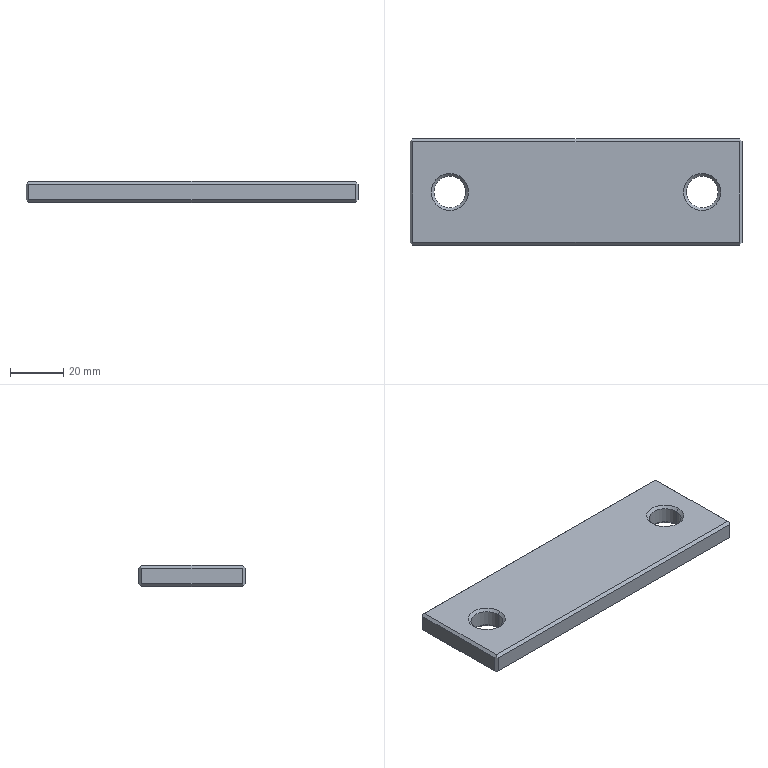Part | SolidWorks | features BaseBody 1 | 1 solid | 30 faces | box 125 x 40 x 8 mm | volume 37771 mm3 | plane 18 | cone 8 | cylinder 4 | commonest cylinder face diameters 12 x4
STEP:
#1=CARTESIAN_POINT('',(53.5,0.,1.));
#2=VERTEX_POINT('',#1);
#3=CARTESIAN_POINT('',(41.5,0.,1.));
#4=VERTEX_POINT('',#3);
#5=CARTESIAN_POINT('',(47.5,0.,1.));
#6=DIRECTION('',(0.,0.,-1.));
#7=DIRECTION('',(0.,-1.,0.));
#8=AXIS2_PLACEMENT_3D('',#5,#6,#7);
#9=CIRCLE('',#8,6.);
#10=EDGE_CURVE('',#2,#4,#9,.T.);
#11=ORIENTED_EDGE('',*,*,#10,.F.);
#12=CARTESIAN_POINT('',(54.5,0.,0.));
#13=VERTEX_POINT('',#12);
#14=CARTESIAN_POINT('',(54.5,0.,0.));
#15=DIRECTION('',(0.7071,0.,-0.7071));
#16=VECTOR('',#15,1000.);
#17=LINE('',#14,#16);
#18=EDGE_CURVE('',#2,#13,#17,.T.);
#19=ORIENTED_EDGE('',*,*,#18,.T.);
#20=CARTESIAN_POINT('',(40.5,0.,0.));
#21=VERTEX_POINT('',#20);
#22=CARTESIAN_POINT('',(47.5,0.,0.));
#23=DIRECTION('',(0.,0.,-1.));
#24=DIRECTION('',(-1.,0.,0.));
#25=AXIS2_PLACEMENT_3D('',#22,#23,#24);
#26=CIRCLE('',#25,7.);
#27=EDGE_CURVE('',#13,#21,#26,.T.);
#28=ORIENTED_EDGE('',*,*,#27,.T.);
#29=CARTESIAN_POINT('',(40.5,0.,0.));
#30=DIRECTION('',(-0.7071,0.,-0.7071));
#31=VECTOR('',#30,1000.);
#32=LINE('',#29,#31);
#33=EDGE_CURVE('',#4,#21,#32,.T.);
#34=ORIENTED_EDGE('',*,*,#33,.F.);
#35=EDGE_LOOP('',(#11,#19,#28,#34));
#36=FACE_OUTER_BOUND('',#35,.T.);
#37=CARTESIAN_POINT('',(47.5,0.,0.));
#38=DIRECTION('',(0.,0.,-1.));
#39=DIRECTION('',(-1.,0.,0.));
#40=AXIS2_PLACEMENT_3D('',#37,#38,#39);
#41=CONICAL_SURFACE('',#40,7.,0.7854);
#42=ADVANCED_FACE('',(#36),#41,.F.);
#43=CARTESIAN_POINT('',(-41.5,0.,1.));
#44=VERTEX_POINT('',#43);
#45=CARTESIAN_POINT('',(-53.5,0.,1.));
#46=VERTEX_POINT('',#45);
#47=CARTESIAN_POINT('',(-47.5,0.,1.));
#48=DIRECTION('',(0.,0.,-1.));
#49=DIRECTION('',(0.,-1.,0.));
#50=AXIS2_PLACEMENT_3D('',#47,#48,#49);
#51=CIRCLE('',#50,6.);
#52=EDGE_CURVE('',#44,#46,#51,.T.);
#53=ORIENTED_EDGE('',*,*,#52,.F.);
#54=CARTESIAN_POINT('',(-40.5,0.,0.));
#55=VERTEX_POINT('',#54);
#56=CARTESIAN_POINT('',(-40.5,0.,0.));
#57=DIRECTION('',(0.7071,0.,-0.7071));
#58=VECTOR('',#57,1000.);
#59=LINE('',#56,#58);
#60=EDGE_CURVE('',#44,#55,#59,.T.);
#61=ORIENTED_EDGE('',*,*,#60,.T.);
#62=CARTESIAN_POINT('',(-54.5,0.,0.));
#63=VERTEX_POINT('',#62);
#64=CARTESIAN_POINT('',(-47.5,0.,0.));
#65=DIRECTION('',(0.,0.,-1.));
#66=DIRECTION('',(-1.,0.,0.));
#67=AXIS2_PLACEMENT_3D('',#64,#65,#66);
#68=CIRCLE('',#67,7.);
#69=EDGE_CURVE('',#55,#63,#68,.T.);
#70=ORIENTED_EDGE('',*,*,#69,.T.);
#71=CARTESIAN_POINT('',(-54.5,0.,0.));
#72=DIRECTION('',(-0.7071,0.,-0.7071));
#73=VECTOR('',#72,1000.);
#74=LINE('',#71,#73);
#75=EDGE_CURVE('',#46,#63,#74,.T.);
#76=ORIENTED_EDGE('',*,*,#75,.F.);
#77=EDGE_LOOP('',(#53,#61,#70,#76));
#78=FACE_OUTER_BOUND('',#77,.T.);
#79=CARTESIAN_POINT('',(-47.5,0.,0.));
#80=DIRECTION('',(0.,0.,-1.));
#81=DIRECTION('',(-1.,0.,0.));
#82=AXIS2_PLACEMENT_3D('',#79,#80,#81);
#83=CONICAL_SURFACE('',#82,7.,0.7854);
#84=ADVANCED_FACE('',(#78),#83,.F.);
#85=CARTESIAN_POINT('',(53.5,0.,7.));
#86=VERTEX_POINT('',#85);
#87=CARTESIAN_POINT('',(41.5,0.,7.));
#88=VERTEX_POINT('',#87);
#89=CARTESIAN_POINT('',(47.5,0.,7.));
#90=DIRECTION('',(0.,0.,-1.));
#91=DIRECTION('',(-1.,0.,0.));
#92=AXIS2_PLACEMENT_3D('',#89,#90,#91);
#93=CIRCLE('',#92,6.);
#94=EDGE_CURVE('',#86,#88,#93,.T.);
#95=ORIENTED_EDGE('',*,*,#94,.F.);
#96=CARTESIAN_POINT('',(53.5,0.,8.));
#97=DIRECTION('',(0.,0.,-1.));
#98=VECTOR('',#97,1000.);
#99=LINE('',#96,#98);
#100=EDGE_CURVE('',#86,#2,#99,.T.);
#101=ORIENTED_EDGE('',*,*,#100,.T.);
#102=ORIENTED_EDGE('',*,*,#10,.T.);
#103=CARTESIAN_POINT('',(41.5,0.,8.));
#104=DIRECTION('',(0.,0.,-1.));
#105=VECTOR('',#104,1000.);
#106=LINE('',#103,#105);
#107=EDGE_CURVE('',#88,#4,#106,.T.);
#108=ORIENTED_EDGE('',*,*,#107,.F.);
#109=EDGE_LOOP('',(#95,#101,#102,#108));
#110=FACE_OUTER_BOUND('',#109,.T.);
#111=CARTESIAN_POINT('',(47.5,0.,8.));
#112=DIRECTION('',(0.,0.,-1.));
#113=DIRECTION('',(-1.,0.,0.));
#114=AXIS2_PLACEMENT_3D('',#111,#112,#113);
#115=CYLINDRICAL_SURFACE('',#114,6.);
#116=ADVANCED_FACE('',(#110),#115,.F.);
#117=CARTESIAN_POINT('',(-41.5,0.,7.));
#118=VERTEX_POINT('',#117);
#119=CARTESIAN_POINT('',(-53.5,0.,7.));
#120=VERTEX_POINT('',#119);
#121=CARTESIAN_POINT('',(-47.5,0.,7.));
#122=DIRECTION('',(0.,0.,-1.));
#123=DIRECTION('',(-1.,0.,0.));
#124=AXIS2_PLACEMENT_3D('',#121,#122,#123);
#125=CIRCLE('',#124,6.);
#126=EDGE_CURVE('',#118,#120,#125,.T.);
#127=ORIENTED_EDGE('',*,*,#126,.F.);
#128=CARTESIAN_POINT('',(-41.5,0.,8.));
#129=DIRECTION('',(0.,0.,-1.));
#130=VECTOR('',#129,1000.);
#131=LINE('',#128,#130);
#132=EDGE_CURVE('',#118,#44,#131,.T.);
#133=ORIENTED_EDGE('',*,*,#132,.T.);
#134=ORIENTED_EDGE('',*,*,#52,.T.);
#135=CARTESIAN_POINT('',(-53.5,0.,8.));
#136=DIRECTION('',(0.,0.,-1.));
#137=VECTOR('',#136,1000.);
#138=LINE('',#135,#137);
#139=EDGE_CURVE('',#120,#46,#138,.T.);
#140=ORIENTED_EDGE('',*,*,#139,.F.);
#141=EDGE_LOOP('',(#127,#133,#134,#140));
#142=FACE_OUTER_BOUND('',#141,.T.);
#143=CARTESIAN_POINT('',(-47.5,0.,8.));
#144=DIRECTION('',(0.,0.,-1.));
#145=DIRECTION('',(-1.,0.,0.));
#146=AXIS2_PLACEMENT_3D('',#143,#144,#145);
#147=CYLINDRICAL_SURFACE('',#146,6.);
#148=ADVANCED_FACE('',(#142),#147,.F.);
#149=ORIENTED_EDGE('',*,*,#94,.T.);
#150=CARTESIAN_POINT('',(40.5,0.,8.));
#151=VERTEX_POINT('',#150);
#152=CARTESIAN_POINT('',(40.5,0.,8.));
#153=DIRECTION('',(-0.7071,0.,0.7071));
#154=VECTOR('',#153,1000.);
#155=LINE('',#152,#154);
#156=EDGE_CURVE('',#88,#151,#155,.T.);
#157=ORIENTED_EDGE('',*,*,#156,.T.);
#158=CARTESIAN_POINT('',(54.5,0.,8.));
#159=VERTEX_POINT('',#158);
#160=CARTESIAN_POINT('',(47.5,0.,8.));
#161=DIRECTION('',(0.,0.,-1.));
#162=DIRECTION('',(1.,0.,0.));
#163=AXIS2_PLACEMENT_3D('',#160,#161,#162);
#164=CIRCLE('',#163,7.);
#165=EDGE_CURVE('',#159,#151,#164,.T.);
#166=ORIENTED_EDGE('',*,*,#165,.F.);
#167=CARTESIAN_POINT('',(54.5,0.,8.));
#168=DIRECTION('',(0.7071,0.,0.7071));
#169=VECTOR('',#168,1000.);
#170=LINE('',#167,#169);
#171=EDGE_CURVE('',#86,#159,#170,.T.);
#172=ORIENTED_EDGE('',*,*,#171,.F.);
#173=EDGE_LOOP('',(#149,#157,#166,#172));
#174=FACE_OUTER_BOUND('',#173,.T.);
#175=CARTESIAN_POINT('',(47.5,0.,8.));
#176=DIRECTION('',(0.,0.,1.));
#177=DIRECTION('',(1.,0.,0.));
#178=AXIS2_PLACEMENT_3D('',#175,#176,#177);
#179=CONICAL_SURFACE('',#178,7.,0.7854);
#180=ADVANCED_FACE('',(#174),#179,.F.);
#181=ORIENTED_EDGE('',*,*,#126,.T.);
#182=CARTESIAN_POINT('',(-54.5,0.,8.));
#183=VERTEX_POINT('',#182);
#184=CARTESIAN_POINT('',(-54.5,0.,8.));
#185=DIRECTION('',(-0.7071,0.,0.7071));
#186=VECTOR('',#185,1000.);
#187=LINE('',#184,#186);
#188=EDGE_CURVE('',#120,#183,#187,.T.);
#189=ORIENTED_EDGE('',*,*,#188,.T.);
#190=CARTESIAN_POINT('',(-40.5,0.,8.));
#191=VERTEX_POINT('',#190);
#192=CARTESIAN_POINT('',(-47.5,0.,8.));
#193=DIRECTION('',(0.,0.,-1.));
#194=DIRECTION('',(1.,0.,0.));
#195=AXIS2_PLACEMENT_3D('',#192,#193,#194);
#196=CIRCLE('',#195,7.);
#197=EDGE_CURVE('',#191,#183,#196,.T.);
#198=ORIENTED_EDGE('',*,*,#197,.F.);
#199=CARTESIAN_POINT('',(-40.5,0.,8.));
#200=DIRECTION('',(0.7071,0.,0.7071));
#201=VECTOR('',#200,1000.);
#202=LINE('',#199,#201);
#203=EDGE_CURVE('',#118,#191,#202,.T.);
#204=ORIENTED_EDGE('',*,*,#203,.F.);
#205=EDGE_LOOP('',(#181,#189,#198,#204));
#206=FACE_OUTER_BOUND('',#205,.T.);
#207=CARTESIAN_POINT('',(-47.5,0.,8.));
#208=DIRECTION('',(0.,0.,1.));
#209=DIRECTION('',(1.,0.,0.));
#210=AXIS2_PLACEMENT_3D('',#207,#208,#209);
#211=CONICAL_SURFACE('',#210,7.,0.7854);
#212=ADVANCED_FACE('',(#206),#211,.F.);
#213=CARTESIAN_POINT('',(47.5,0.,0.));
#214=DIRECTION('',(0.,0.,-1.));
#215=DIRECTION('',(-1.,0.,0.));
#216=AXIS2_PLACEMENT_3D('',#213,#214,#215);
#217=CIRCLE('',#216,7.);
#218=EDGE_CURVE('',#21,#13,#217,.T.);
#219=ORIENTED_EDGE('',*,*,#218,.F.);
#220=ORIENTED_EDGE('',*,*,#27,.F.);
#221=EDGE_LOOP('',(#219,#220));
#222=FACE_BOUND('',#221,.T.);
#223=CARTESIAN_POINT('',(-47.5,0.,0.));
#224=DIRECTION('',(0.,0.,-1.));
#225=DIRECTION('',(-1.,0.,0.));
#226=AXIS2_PLACEMENT_3D('',#223,#224,#225);
#227=CIRCLE('',#226,7.);
#228=EDGE_CURVE('',#63,#55,#227,.T.);
#229=ORIENTED_EDGE('',*,*,#228,.F.);
#230=ORIENTED_EDGE('',*,*,#69,.F.);
#231=EDGE_LOOP('',(#229,#230));
#232=FACE_BOUND('',#231,.T.);
#233=CARTESIAN_POINT('',(-61.5,-19.,0.));
#234=VERTEX_POINT('',#233);
#235=CARTESIAN_POINT('',(61.5,-19.,0.));
#236=VERTEX_POINT('',#235);
#237=CARTESIAN_POINT('',(0.,-19.,0.));
#238=DIRECTION('',(1.,0.,0.));
#239=VECTOR('',#238,1000.);
#240=LINE('',#237,#239);
#241=EDGE_CURVE('',#234,#236,#240,.T.);
#242=ORIENTED_EDGE('',*,*,#241,.F.);
#243=CARTESIAN_POINT('',(-61.5,19.,0.));
#244=VERTEX_POINT('',#243);
#245=CARTESIAN_POINT('',(-61.5,0.,0.));
#246=DIRECTION('',(0.,-1.,0.));
#247=VECTOR('',#246,1000.);
#248=LINE('',#245,#247);
#249=EDGE_CURVE('',#244,#234,#248,.T.);
#250=ORIENTED_EDGE('',*,*,#249,.F.);
#251=CARTESIAN_POINT('',(61.5,19.,0.));
#252=VERTEX_POINT('',#251);
#253=CARTESIAN_POINT('',(0.,19.,0.));
#254=DIRECTION('',(-1.,0.,0.));
#255=VECTOR('',#254,1000.);
#256=LINE('',#253,#255);
#257=EDGE_CURVE('',#252,#244,#256,.T.);
#258=ORIENTED_EDGE('',*,*,#257,.F.);
#259=CARTESIAN_POINT('',(61.5,0.,0.));
#260=DIRECTION('',(0.,1.,0.));
#261=VECTOR('',#260,1000.);
#262=LINE('',#259,#261);
#263=EDGE_CURVE('',#236,#252,#262,.T.);
#264=ORIENTED_EDGE('',*,*,#263,.F.);
#265=EDGE_LOOP('',(#242,#250,#258,#264));
#266=FACE_OUTER_BOUND('',#265,.T.);
#267=CARTESIAN_POINT('',(0.,0.,0.));
#268=DIRECTION('',(0.,0.,1.));
#269=DIRECTION('',(1.,0.,0.));
#270=AXIS2_PLACEMENT_3D('',#267,#268,#269);
#271=PLANE('',#270);
#272=ADVANCED_FACE('',(#222,#232,#266),#271,.F.);
#273=ORIENTED_EDGE('',*,*,#18,.F.);
#274=CARTESIAN_POINT('',(47.5,0.,1.));
#275=DIRECTION('',(0.,0.,-1.));
#276=DIRECTION('',(0.,-1.,0.));
#277=AXIS2_PLACEMENT_3D('',#274,#275,#276);
#278=CIRCLE('',#277,6.);
#279=EDGE_CURVE('',#4,#2,#278,.T.);
#280=ORIENTED_EDGE('',*,*,#279,.F.);
#281=ORIENTED_EDGE('',*,*,#33,.T.);
#282=ORIENTED_EDGE('',*,*,#218,.T.);
#283=EDGE_LOOP('',(#273,#280,#281,#282));
#284=FACE_OUTER_BOUND('',#283,.T.);
#285=CARTESIAN_POINT('',(47.5,0.,0.));
#286=DIRECTION('',(0.,0.,-1.));
#287=DIRECTION('',(-1.,0.,0.));
#288=AXIS2_PLACEMENT_3D('',#285,#286,#287);
#289=CONICAL_SURFACE('',#288,7.,0.7854);
#290=ADVANCED_FACE('',(#284),#289,.F.);
#291=ORIENTED_EDGE('',*,*,#60,.F.);
#292=CARTESIAN_POINT('',(-47.5,0.,1.));
#293=DIRECTION('',(0.,0.,-1.));
#294=DIRECTION('',(0.,-1.,0.));
#295=AXIS2_PLACEMENT_3D('',#292,#293,#294);
#296=CIRCLE('',#295,6.);
#297=EDGE_CURVE('',#46,#44,#296,.T.);
#298=ORIENTED_EDGE('',*,*,#297,.F.);
#299=ORIENTED_EDGE('',*,*,#75,.T.);
#300=ORIENTED_EDGE('',*,*,#228,.T.);
#301=EDGE_LOOP('',(#291,#298,#299,#300));
#302=FACE_OUTER_BOUND('',#301,.T.);
#303=CARTESIAN_POINT('',(-47.5,0.,0.));
#304=DIRECTION('',(0.,0.,-1.));
#305=DIRECTION('',(-1.,0.,0.));
#306=AXIS2_PLACEMENT_3D('',#303,#304,#305);
#307=CONICAL_SURFACE('',#306,7.,0.7854);
#308=ADVANCED_FACE('',(#302),#307,.F.);
#309=CARTESIAN_POINT('',(62.,-19.5,0.5));
#310=VERTEX_POINT('',#309);
#311=CARTESIAN_POINT('',(62.,-19.5,0.5));
#312=DIRECTION('',(-0.5774,0.5774,-0.5774));
#313=VECTOR('',#312,1000.);
#314=LINE('',#311,#313);
#315=EDGE_CURVE('',#310,#236,#314,.T.);
#316=ORIENTED_EDGE('',*,*,#315,.T.);
#317=ORIENTED_EDGE('',*,*,#263,.T.);
#318=CARTESIAN_POINT('',(62.,19.5,0.5));
#319=VERTEX_POINT('',#318);
#320=CARTESIAN_POINT('',(61.5,19.,0.));
#321=DIRECTION('',(0.5774,0.5774,0.5774));
#322=VECTOR('',#321,1000.);
#323=LINE('',#320,#322);
#324=EDGE_CURVE('',#252,#319,#323,.T.);
#325=ORIENTED_EDGE('',*,*,#324,.T.);
#326=CARTESIAN_POINT('',(62.5,19.,1.));
#327=VERTEX_POINT('',#326);
#328=CARTESIAN_POINT('',(62.5,19.,1.));
#329=DIRECTION('',(-0.5774,0.5774,-0.5774));
#330=VECTOR('',#329,1000.);
#331=LINE('',#328,#330);
#332=EDGE_CURVE('',#327,#319,#331,.T.);
#333=ORIENTED_EDGE('',*,*,#332,.F.);
#334=CARTESIAN_POINT('',(62.5,-19.,1.));
#335=VERTEX_POINT('',#334);
#336=CARTESIAN_POINT('',(62.5,0.,1.));
#337=DIRECTION('',(0.,-1.,0.));
#338=VECTOR('',#337,1000.);
#339=LINE('',#336,#338);
#340=EDGE_CURVE('',#327,#335,#339,.T.);
#341=ORIENTED_EDGE('',*,*,#340,.T.);
#342=CARTESIAN_POINT('',(62.,-19.5,0.5));
#343=DIRECTION('',(0.5774,0.5774,0.5774));
#344=VECTOR('',#343,1000.);
#345=LINE('',#342,#344);
#346=EDGE_CURVE('',#310,#335,#345,.T.);
#347=ORIENTED_EDGE('',*,*,#346,.F.);
#348=EDGE_LOOP('',(#316,#317,#325,#333,#341,#347));
#349=FACE_OUTER_BOUND('',#348,.T.);
#350=CARTESIAN_POINT('',(62.,0.,0.5));
#351=DIRECTION('',(0.7071,0.,-0.7071));
#352=DIRECTION('',(-0.7071,0.,-0.7071));
#353=AXIS2_PLACEMENT_3D('',#350,#351,#352);
#354=PLANE('',#353);
#355=ADVANCED_FACE('',(#349),#354,.T.);
#356=CARTESIAN_POINT('',(-62.,-19.5,0.5));
#357=VERTEX_POINT('',#356);
#358=CARTESIAN_POINT('',(-62.,-19.5,0.5));
#359=DIRECTION('',(0.5774,0.5774,-0.5774));
#360=VECTOR('',#359,1000.);
#361=LINE('',#358,#360);
#362=EDGE_CURVE('',#357,#234,#361,.T.);
#363=ORIENTED_EDGE('',*,*,#362,.T.);
#364=ORIENTED_EDGE('',*,*,#241,.T.);
#365=ORIENTED_EDGE('',*,*,#315,.F.);
#366=CARTESIAN_POINT('',(61.5,-20.,1.));
#367=VERTEX_POINT('',#366);
#368=CARTESIAN_POINT('',(61.5,-20.,1.));
#369=DIRECTION('',(0.5774,0.5774,-0.5774));
#370=VECTOR('',#369,1000.);
#371=LINE('',#368,#370);
#372=EDGE_CURVE('',#367,#310,#371,.T.);
#373=ORIENTED_EDGE('',*,*,#372,.F.);
#374=CARTESIAN_POINT('',(-61.5,-20.,1.));
#375=VERTEX_POINT('',#374);
#376=CARTESIAN_POINT('',(0.,-20.,1.));
#377=DIRECTION('',(-1.,0.,0.));
#378=VECTOR('',#377,1000.);
#379=LINE('',#376,#378);
#380=EDGE_CURVE('',#367,#375,#379,.T.);
#381=ORIENTED_EDGE('',*,*,#380,.T.);
#382=CARTESIAN_POINT('',(-62.,-19.5,0.5));
#383=DIRECTION('',(0.5774,-0.5774,0.5774));
#384=VECTOR('',#383,1000.);
#385=LINE('',#382,#384);
#386=EDGE_CURVE('',#357,#375,#385,.T.);
#387=ORIENTED_EDGE('',*,*,#386,.F.);
#388=EDGE_LOOP('',(#363,#364,#365,#373,#381,#387));
#389=FACE_OUTER_BOUND('',#388,.T.);
#390=CARTESIAN_POINT('',(0.,-19.5,0.5));
#391=DIRECTION('',(0.,-0.7071,-0.7071));
#392=DIRECTION('',(0.,0.7071,-0.7071));
#393=AXIS2_PLACEMENT_3D('',#390,#391,#392);
#394=PLANE('',#393);
#395=ADVANCED_FACE('',(#389),#394,.T.);
#396=CARTESIAN_POINT('',(-62.5,-19.,1.));
#397=VERTEX_POINT('',#396);
#398=CARTESIAN_POINT('',(-62.5,-19.,1.));
#399=DIRECTION('',(0.5774,-0.5774,-0.5774));
#400=VECTOR('',#399,1000.);
#401=LINE('',#398,#400);
#402=EDGE_CURVE('',#397,#357,#401,.T.);
#403=ORIENTED_EDGE('',*,*,#402,.F.);
#404=CARTESIAN_POINT('',(-62.5,19.,1.));
#405=VERTEX_POINT('',#404);
#406=CARTESIAN_POINT('',(-62.5,0.,1.));
#407=DIRECTION('',(0.,1.,0.));
#408=VECTOR('',#407,1000.);
#409=LINE('',#406,#408);
#410=EDGE_CURVE('',#397,#405,#409,.T.);
#411=ORIENTED_EDGE('',*,*,#410,.T.);
#412=CARTESIAN_POINT('',(-62.,19.5,0.5));
#413=VERTEX_POINT('',#412);
#414=CARTESIAN_POINT('',(-62.,19.5,0.5));
#415=DIRECTION('',(-0.5774,-0.5774,0.5774));
#416=VECTOR('',#415,1000.);
#417=LINE('',#414,#416);
#418=EDGE_CURVE('',#413,#405,#417,.T.);
#419=ORIENTED_EDGE('',*,*,#418,.F.);
#420=CARTESIAN_POINT('',(-62.,19.5,0.5));
#421=DIRECTION('',(0.5774,-0.5774,-0.5774));
#422=VECTOR('',#421,1000.);
#423=LINE('',#420,#422);
#424=EDGE_CURVE('',#413,#244,#423,.T.);
#425=ORIENTED_EDGE('',*,*,#424,.T.);
#426=ORIENTED_EDGE('',*,*,#249,.T.);
#427=ORIENTED_EDGE('',*,*,#362,.F.);
#428=EDGE_LOOP('',(#403,#411,#419,#425,#426,#427));
#429=FACE_OUTER_BOUND('',#428,.T.);
#430=CARTESIAN_POINT('',(-62.,0.,0.5));
#431=DIRECTION('',(-0.7071,0.,-0.7071));
#432=DIRECTION('',(-0.7071,0.,0.7071));
#433=AXIS2_PLACEMENT_3D('',#430,#431,#432);
#434=PLANE('',#433);
#435=ADVANCED_FACE('',(#429),#434,.T.);
#436=CARTESIAN_POINT('',(-61.5,20.,1.));
#437=VERTEX_POINT('',#436);
#438=CARTESIAN_POINT('',(-61.5,20.,1.));
#439=DIRECTION('',(-0.5774,-0.5774,-0.5774));
#440=VECTOR('',#439,1000.);
#441=LINE('',#438,#440);
#442=EDGE_CURVE('',#437,#413,#441,.T.);
#443=ORIENTED_EDGE('',*,*,#442,.F.);
#444=CARTESIAN_POINT('',(61.5,20.,1.));
#445=VERTEX_POINT('',#444);
#446=CARTESIAN_POINT('',(0.,20.,1.));
#447=DIRECTION('',(1.,0.,0.));
#448=VECTOR('',#447,1000.);
#449=LINE('',#446,#448);
#450=EDGE_CURVE('',#437,#445,#449,.T.);
#451=ORIENTED_EDGE('',*,*,#450,.T.);
#452=CARTESIAN_POINT('',(62.,19.5,0.5));
#453=DIRECTION('',(-0.5774,0.5774,0.5774));
#454=VECTOR('',#453,1000.);
#455=LINE('',#452,#454);
#456=EDGE_CURVE('',#319,#445,#455,.T.);
#457=ORIENTED_EDGE('',*,*,#456,.F.);
#458=ORIENTED_EDGE('',*,*,#324,.F.);
#459=ORIENTED_EDGE('',*,*,#257,.T.);
#460=ORIENTED_EDGE('',*,*,#424,.F.);
#461=EDGE_LOOP('',(#443,#451,#457,#458,#459,#460));
#462=FACE_OUTER_BOUND('',#461,.T.);
#463=CARTESIAN_POINT('',(0.,19.5,0.5));
#464=DIRECTION('',(0.,0.7071,-0.7071));
#465=DIRECTION('',(0.,0.7071,0.7071));
#466=AXIS2_PLACEMENT_3D('',#463,#464,#465);
#467=PLANE('',#466);
#468=ADVANCED_FACE('',(#462),#467,.T.);
#469=ORIENTED_EDGE('',*,*,#100,.F.);
#470=CARTESIAN_POINT('',(47.5,0.,7.));
#471=DIRECTION('',(0.,0.,-1.));
#472=DIRECTION('',(-1.,0.,0.));
#473=AXIS2_PLACEMENT_3D('',#470,#471,#472);
#474=CIRCLE('',#473,6.);
#475=EDGE_CURVE('',#88,#86,#474,.T.);
#476=ORIENTED_EDGE('',*,*,#475,.F.);
#477=ORIENTED_EDGE('',*,*,#107,.T.);
#478=ORIENTED_EDGE('',*,*,#279,.T.);
#479=EDGE_LOOP('',(#469,#476,#477,#478));
#480=FACE_OUTER_BOUND('',#479,.T.);
#481=CARTESIAN_POINT('',(47.5,0.,8.));
#482=DIRECTION('',(0.,0.,-1.));
#483=DIRECTION('',(-1.,0.,0.));
#484=AXIS2_PLACEMENT_3D('',#481,#482,#483);
#485=CYLINDRICAL_SURFACE('',#484,6.);
#486=ADVANCED_FACE('',(#480),#485,.F.);
#487=ORIENTED_EDGE('',*,*,#132,.F.);
#488=CARTESIAN_POINT('',(-47.5,0.,7.));
#489=DIRECTION('',(0.,0.,-1.));
#490=DIRECTION('',(-1.,0.,0.));
#491=AXIS2_PLACEMENT_3D('',#488,#489,#490);
#492=CIRCLE('',#491,6.);
#493=EDGE_CURVE('',#120,#118,#492,.T.);
#494=ORIENTED_EDGE('',*,*,#493,.F.);
#495=ORIENTED_EDGE('',*,*,#139,.T.);
#496=ORIENTED_EDGE('',*,*,#297,.T.);
#497=EDGE_LOOP('',(#487,#494,#495,#496));
#498=FACE_OUTER_BOUND('',#497,.T.);
#499=CARTESIAN_POINT('',(-47.5,0.,8.));
#500=DIRECTION('',(0.,0.,-1.));
#501=DIRECTION('',(-1.,0.,0.));
#502=AXIS2_PLACEMENT_3D('',#499,#500,#501);
#503=CYLINDRICAL_SURFACE('',#502,6.);
#504=ADVANCED_FACE('',(#498),#503,.F.);
#505=CARTESIAN_POINT('',(62.5,19.,7.));
#506=VERTEX_POINT('',#505);
#507=CARTESIAN_POINT('',(62.5,-19.,7.));
#508=VERTEX_POINT('',#507);
#509=CARTESIAN_POINT('',(62.5,-20.,7.));
#510=DIRECTION('',(0.,-1.,0.));
#511=VECTOR('',#510,1000.);
#512=LINE('',#509,#511);
#513=EDGE_CURVE('',#506,#508,#512,.T.);
#514=ORIENTED_EDGE('',*,*,#513,.T.);
#515=CARTESIAN_POINT('',(62.5,-19.,0.));
#516=DIRECTION('',(0.,0.,-1.));
#517=VECTOR('',#516,1000.);
#518=LINE('',#515,#517);
#519=EDGE_CURVE('',#508,#335,#518,.T.);
#520=ORIENTED_EDGE('',*,*,#519,.T.);
#521=ORIENTED_EDGE('',*,*,#340,.F.);
#522=CARTESIAN_POINT('',(62.5,19.,0.));
#523=DIRECTION('',(0.,0.,1.));
#524=VECTOR('',#523,1000.);
#525=LINE('',#522,#524);
#526=EDGE_CURVE('',#327,#506,#525,.T.);
#527=ORIENTED_EDGE('',*,*,#526,.T.);
#528=EDGE_LOOP('',(#514,#520,#521,#527));
#529=FACE_OUTER_BOUND('',#528,.T.);
#530=CARTESIAN_POINT('',(62.5,-20.,0.));
#531=DIRECTION('',(1.,0.,0.));
#532=DIRECTION('',(0.,0.,-1.));
#533=AXIS2_PLACEMENT_3D('',#530,#531,#532);
#534=PLANE('',#533);
#535=ADVANCED_FACE('',(#529),#534,.T.);
#536=CARTESIAN_POINT('',(61.5,-20.,7.));
#537=VERTEX_POINT('',#536);
#538=CARTESIAN_POINT('',(-61.5,-20.,7.));
#539=VERTEX_POINT('',#538);
#540=CARTESIAN_POINT('',(-62.5,-20.,7.));
#541=DIRECTION('',(-1.,0.,0.));
#542=VECTOR('',#541,1000.);
#543=LINE('',#540,#542);
#544=EDGE_CURVE('',#537,#539,#543,.T.);
#545=ORIENTED_EDGE('',*,*,#544,.T.);
#546=CARTESIAN_POINT('',(-61.5,-20.,0.));
#547=DIRECTION('',(0.,0.,-1.));
#548=VECTOR('',#547,1000.);
#549=LINE('',#546,#548);
#550=EDGE_CURVE('',#539,#375,#549,.T.);
#551=ORIENTED_EDGE('',*,*,#550,.T.);
#552=ORIENTED_EDGE('',*,*,#380,.F.);
#553=CARTESIAN_POINT('',(61.5,-20.,0.));
#554=DIRECTION('',(0.,0.,1.));
#555=VECTOR('',#554,1000.);
#556=LINE('',#553,#555);
#557=EDGE_CURVE('',#367,#537,#556,.T.);
#558=ORIENTED_EDGE('',*,*,#557,.T.);
#559=EDGE_LOOP('',(#545,#551,#552,#558));
#560=FACE_OUTER_BOUND('',#559,.T.);
#561=CARTESIAN_POINT('',(-62.5,-20.,0.));
#562=DIRECTION('',(0.,-1.,0.));
#563=DIRECTION('',(0.,0.,-1.));
#564=AXIS2_PLACEMENT_3D('',#561,#562,#563);
#565=PLANE('',#564);
#566=ADVANCED_FACE('',(#560),#565,.T.);
#567=CARTESIAN_POINT('',(-62.5,-19.,7.));
#568=VERTEX_POINT('',#567);
#569=CARTESIAN_POINT('',(-62.5,-19.,0.));
#570=DIRECTION('',(0.,0.,1.));
#571=VECTOR('',#570,1000.);
#572=LINE('',#569,#571);
#573=EDGE_CURVE('',#397,#568,#572,.T.);
#574=ORIENTED_EDGE('',*,*,#573,.T.);
#575=CARTESIAN_POINT('',(-62.5,19.,7.));
#576=VERTEX_POINT('',#575);
#577=CARTESIAN_POINT('',(-62.5,20.,7.));
#578=DIRECTION('',(0.,1.,0.));
#579=VECTOR('',#578,1000.);
#580=LINE('',#577,#579);
#581=EDGE_CURVE('',#568,#576,#580,.T.);
#582=ORIENTED_EDGE('',*,*,#581,.T.);
#583=CARTESIAN_POINT('',(-62.5,19.,0.));
#584=DIRECTION('',(0.,0.,-1.));
#585=VECTOR('',#584,1000.);
#586=LINE('',#583,#585);
#587=EDGE_CURVE('',#576,#405,#586,.T.);
#588=ORIENTED_EDGE('',*,*,#587,.T.);
#589=ORIENTED_EDGE('',*,*,#410,.F.);
#590=EDGE_LOOP('',(#574,#582,#588,#589));
#591=FACE_OUTER_BOUND('',#590,.T.);
#592=CARTESIAN_POINT('',(-62.5,20.,0.));
#593=DIRECTION('',(-1.,0.,0.));
#594=DIRECTION('',(0.,0.,1.));
#595=AXIS2_PLACEMENT_3D('',#592,#593,#594);
#596=PLANE('',#595);
#597=ADVANCED_FACE('',(#591),#596,.T.);
#598=CARTESIAN_POINT('',(-61.5,20.,7.));
#599=VERTEX_POINT('',#598);
#600=CARTESIAN_POINT('',(61.5,20.,7.));
#601=VERTEX_POINT('',#600);
#602=CARTESIAN_POINT('',(62.5,20.,7.));
#603=DIRECTION('',(1.,0.,0.));
#604=VECTOR('',#603,1000.);
#605=LINE('',#602,#604);
#606=EDGE_CURVE('',#599,#601,#605,.T.);
#607=ORIENTED_EDGE('',*,*,#606,.T.);
#608=CARTESIAN_POINT('',(61.5,20.,0.));
#609=DIRECTION('',(0.,0.,-1.));
#610=VECTOR('',#609,1000.);
#611=LINE('',#608,#610);
#612=EDGE_CURVE('',#601,#445,#611,.T.);
#613=ORIENTED_EDGE('',*,*,#612,.T.);
#614=ORIENTED_EDGE('',*,*,#450,.F.);
#615=CARTESIAN_POINT('',(-61.5,20.,0.));
#616=DIRECTION('',(0.,0.,1.));
#617=VECTOR('',#616,1000.);
#618=LINE('',#615,#617);
#619=EDGE_CURVE('',#437,#599,#618,.T.);
#620=ORIENTED_EDGE('',*,*,#619,.T.);
#621=EDGE_LOOP('',(#607,#613,#614,#620));
#622=FACE_OUTER_BOUND('',#621,.T.);
#623=CARTESIAN_POINT('',(62.5,20.,0.));
#624=DIRECTION('',(0.,1.,0.));
#625=DIRECTION('',(0.,0.,1.));
#626=AXIS2_PLACEMENT_3D('',#623,#624,#625);
#627=PLANE('',#626);
#628=ADVANCED_FACE('',(#622),#627,.T.);
#629=ORIENTED_EDGE('',*,*,#156,.F.);
#630=ORIENTED_EDGE('',*,*,#475,.T.);
#631=ORIENTED_EDGE('',*,*,#171,.T.);
#632=CARTESIAN_POINT('',(47.5,0.,8.));
#633=DIRECTION('',(0.,0.,-1.));
#634=DIRECTION('',(1.,0.,0.));
#635=AXIS2_PLACEMENT_3D('',#632,#633,#634);
#636=CIRCLE('',#635,7.);
#637=EDGE_CURVE('',#151,#159,#636,.T.);
#638=ORIENTED_EDGE('',*,*,#637,.F.);
#639=EDGE_LOOP('',(#629,#630,#631,#638));
#640=FACE_OUTER_BOUND('',#639,.T.);
#641=CARTESIAN_POINT('',(47.5,0.,8.));
#642=DIRECTION('',(0.,0.,1.));
#643=DIRECTION('',(1.,0.,0.));
#644=AXIS2_PLACEMENT_3D('',#641,#642,#643);
#645=CONICAL_SURFACE('',#644,7.,0.7854);
#646=ADVANCED_FACE('',(#640),#645,.F.);
#647=ORIENTED_EDGE('',*,*,#188,.F.);
#648=ORIENTED_EDGE('',*,*,#493,.T.);
#649=ORIENTED_EDGE('',*,*,#203,.T.);
#650=CARTESIAN_POINT('',(-47.5,0.,8.));
#651=DIRECTION('',(0.,0.,-1.));
#652=DIRECTION('',(1.,0.,0.));
#653=AXIS2_PLACEMENT_3D('',#650,#651,#652);
#654=CIRCLE('',#653,7.);
#655=EDGE_CURVE('',#183,#191,#654,.T.);
#656=ORIENTED_EDGE('',*,*,#655,.F.);
#657=EDGE_LOOP('',(#647,#648,#649,#656));
#658=FACE_OUTER_BOUND('',#657,.T.);
#659=CARTESIAN_POINT('',(-47.5,0.,8.));
#660=DIRECTION('',(0.,0.,1.));
#661=DIRECTION('',(1.,0.,0.));
#662=AXIS2_PLACEMENT_3D('',#659,#660,#661);
#663=CONICAL_SURFACE('',#662,7.,0.7854);
#664=ADVANCED_FACE('',(#658),#663,.F.);
#665=ORIENTED_EDGE('',*,*,#346,.T.);
#666=ORIENTED_EDGE('',*,*,#519,.F.);
#667=CARTESIAN_POINT('',(62.,-19.5,7.5));
#668=VERTEX_POINT('',#667);
#669=CARTESIAN_POINT('',(62.5,-19.,7.));
#670=DIRECTION('',(-0.5774,-0.5774,0.5774));
#671=VECTOR('',#670,1000.);
#672=LINE('',#669,#671);
#673=EDGE_CURVE('',#508,#668,#672,.T.);
#674=ORIENTED_EDGE('',*,*,#673,.T.);
#675=CARTESIAN_POINT('',(62.,-19.5,7.5));
#676=DIRECTION('',(-0.5774,-0.5774,-0.5774));
#677=VECTOR('',#676,1000.);
#678=LINE('',#675,#677);
#679=EDGE_CURVE('',#668,#537,#678,.T.);
#680=ORIENTED_EDGE('',*,*,#679,.T.);
#681=ORIENTED_EDGE('',*,*,#557,.F.);
#682=ORIENTED_EDGE('',*,*,#372,.T.);
#683=EDGE_LOOP('',(#665,#666,#674,#680,#681,#682));
#684=FACE_OUTER_BOUND('',#683,.T.);
#685=CARTESIAN_POINT('',(62.,-19.5,4.));
#686=DIRECTION('',(0.7071,-0.7071,0.));
#687=DIRECTION('',(0.7071,0.7071,0.));
#688=AXIS2_PLACEMENT_3D('',#685,#686,#687);
#689=PLANE('',#688);
#690=ADVANCED_FACE('',(#684),#689,.T.);
#691=ORIENTED_EDGE('',*,*,#673,.F.);
#692=ORIENTED_EDGE('',*,*,#513,.F.);
#693=CARTESIAN_POINT('',(62.,19.5,7.5));
#694=VERTEX_POINT('',#693);
#695=CARTESIAN_POINT('',(62.5,19.,7.));
#696=DIRECTION('',(-0.5774,0.5774,0.5774));
#697=VECTOR('',#696,1000.);
#698=LINE('',#695,#697);
#699=EDGE_CURVE('',#506,#694,#698,.T.);
#700=ORIENTED_EDGE('',*,*,#699,.T.);
#701=CARTESIAN_POINT('',(61.5,19.,8.));
#702=VERTEX_POINT('',#701);
#703=CARTESIAN_POINT('',(62.,19.5,7.5));
#704=DIRECTION('',(-0.5774,-0.5774,0.5774));
#705=VECTOR('',#704,1000.);
#706=LINE('',#703,#705);
#707=EDGE_CURVE('',#694,#702,#706,.T.);
#708=ORIENTED_EDGE('',*,*,#707,.T.);
#709=CARTESIAN_POINT('',(61.5,-19.,8.));
#710=VERTEX_POINT('',#709);
#711=CARTESIAN_POINT('',(61.5,0.,8.));
#712=DIRECTION('',(0.,-1.,0.));
#713=VECTOR('',#712,1000.);
#714=LINE('',#711,#713);
#715=EDGE_CURVE('',#702,#710,#714,.T.);
#716=ORIENTED_EDGE('',*,*,#715,.T.);
#717=CARTESIAN_POINT('',(61.5,-19.,8.));
#718=DIRECTION('',(0.5774,-0.5774,-0.5774));
#719=VECTOR('',#718,1000.);
#720=LINE('',#717,#719);
#721=EDGE_CURVE('',#710,#668,#720,.T.);
#722=ORIENTED_EDGE('',*,*,#721,.T.);
#723=EDGE_LOOP('',(#691,#692,#700,#708,#716,#722));
#724=FACE_OUTER_BOUND('',#723,.T.);
#725=CARTESIAN_POINT('',(62.,0.,7.5));
#726=DIRECTION('',(0.7071,0.,0.7071));
#727=DIRECTION('',(0.7071,0.,-0.7071));
#728=AXIS2_PLACEMENT_3D('',#725,#726,#727);
#729=PLANE('',#728);
#730=ADVANCED_FACE('',(#724),#729,.T.);
#731=ORIENTED_EDGE('',*,*,#456,.T.);
#732=ORIENTED_EDGE('',*,*,#612,.F.);
#733=CARTESIAN_POINT('',(61.5,20.,7.));
#734=DIRECTION('',(0.5774,-0.5774,0.5774));
#735=VECTOR('',#734,1000.);
#736=LINE('',#733,#735);
#737=EDGE_CURVE('',#601,#694,#736,.T.);
#738=ORIENTED_EDGE('',*,*,#737,.T.);
#739=ORIENTED_EDGE('',*,*,#699,.F.);
#740=ORIENTED_EDGE('',*,*,#526,.F.);
#741=ORIENTED_EDGE('',*,*,#332,.T.);
#742=EDGE_LOOP('',(#731,#732,#738,#739,#740,#741));
#743=FACE_OUTER_BOUND('',#742,.T.);
#744=CARTESIAN_POINT('',(62.,19.5,4.));
#745=DIRECTION('',(0.7071,0.7071,0.));
#746=DIRECTION('',(-0.7071,0.7071,0.));
#747=AXIS2_PLACEMENT_3D('',#744,#745,#746);
#748=PLANE('',#747);
#749=ADVANCED_FACE('',(#743),#748,.T.);
#750=ORIENTED_EDGE('',*,*,#386,.T.);
#751=ORIENTED_EDGE('',*,*,#550,.F.);
#752=CARTESIAN_POINT('',(-62.,-19.5,7.5));
#753=VERTEX_POINT('',#752);
#754=CARTESIAN_POINT('',(-61.5,-20.,7.));
#755=DIRECTION('',(-0.5774,0.5774,0.5774));
#756=VECTOR('',#755,1000.);
#757=LINE('',#754,#756);
#758=EDGE_CURVE('',#539,#753,#757,.T.);
#759=ORIENTED_EDGE('',*,*,#758,.T.);
#760=CARTESIAN_POINT('',(-62.,-19.5,7.5));
#761=DIRECTION('',(-0.5774,0.5774,-0.5774));
#762=VECTOR('',#761,1000.);
#763=LINE('',#760,#762);
#764=EDGE_CURVE('',#753,#568,#763,.T.);
#765=ORIENTED_EDGE('',*,*,#764,.T.);
#766=ORIENTED_EDGE('',*,*,#573,.F.);
#767=ORIENTED_EDGE('',*,*,#402,.T.);
#768=EDGE_LOOP('',(#750,#751,#759,#765,#766,#767));
#769=FACE_OUTER_BOUND('',#768,.T.);
#770=CARTESIAN_POINT('',(-62.,-19.5,4.));
#771=DIRECTION('',(-0.7071,-0.7071,0.));
#772=DIRECTION('',(0.7071,-0.7071,0.));
#773=AXIS2_PLACEMENT_3D('',#770,#771,#772);
#774=PLANE('',#773);
#775=ADVANCED_FACE('',(#769),#774,.T.);
#776=ORIENTED_EDGE('',*,*,#758,.F.);
#777=ORIENTED_EDGE('',*,*,#544,.F.);
#778=ORIENTED_EDGE('',*,*,#679,.F.);
#779=ORIENTED_EDGE('',*,*,#721,.F.);
#780=CARTESIAN_POINT('',(-61.5,-19.,8.));
#781=VERTEX_POINT('',#780);
#782=CARTESIAN_POINT('',(0.,-19.,8.));
#783=DIRECTION('',(-1.,0.,0.));
#784=VECTOR('',#783,1000.);
#785=LINE('',#782,#784);
#786=EDGE_CURVE('',#710,#781,#785,.T.);
#787=ORIENTED_EDGE('',*,*,#786,.T.);
#788=CARTESIAN_POINT('',(-61.5,-19.,8.));
#789=DIRECTION('',(-0.5774,-0.5774,-0.5774));
#790=VECTOR('',#789,1000.);
#791=LINE('',#788,#790);
#792=EDGE_CURVE('',#781,#753,#791,.T.);
#793=ORIENTED_EDGE('',*,*,#792,.T.);
#794=EDGE_LOOP('',(#776,#777,#778,#779,#787,#793));
#795=FACE_OUTER_BOUND('',#794,.T.);
#796=CARTESIAN_POINT('',(0.,-19.5,7.5));
#797=DIRECTION('',(0.,-0.7071,0.7071));
#798=DIRECTION('',(0.,-0.7071,-0.7071));
#799=AXIS2_PLACEMENT_3D('',#796,#797,#798);
#800=PLANE('',#799);
#801=ADVANCED_FACE('',(#795),#800,.T.);
#802=CARTESIAN_POINT('',(-62.,19.5,7.5));
#803=VERTEX_POINT('',#802);
#804=CARTESIAN_POINT('',(-62.,19.5,7.5));
#805=DIRECTION('',(-0.5774,-0.5774,-0.5774));
#806=VECTOR('',#805,1000.);
#807=LINE('',#804,#806);
#808=EDGE_CURVE('',#803,#576,#807,.T.);
#809=ORIENTED_EDGE('',*,*,#808,.T.);
#810=ORIENTED_EDGE('',*,*,#581,.F.);
#811=ORIENTED_EDGE('',*,*,#764,.F.);
#812=ORIENTED_EDGE('',*,*,#792,.F.);
#813=CARTESIAN_POINT('',(-61.5,19.,8.));
#814=VERTEX_POINT('',#813);
#815=CARTESIAN_POINT('',(-61.5,0.,8.));
#816=DIRECTION('',(0.,1.,0.));
#817=VECTOR('',#816,1000.);
#818=LINE('',#815,#817);
#819=EDGE_CURVE('',#781,#814,#818,.T.);
#820=ORIENTED_EDGE('',*,*,#819,.T.);
#821=CARTESIAN_POINT('',(-61.5,19.,8.));
#822=DIRECTION('',(-0.5774,0.5774,-0.5774));
#823=VECTOR('',#822,1000.);
#824=LINE('',#821,#823);
#825=EDGE_CURVE('',#814,#803,#824,.T.);
#826=ORIENTED_EDGE('',*,*,#825,.T.);
#827=EDGE_LOOP('',(#809,#810,#811,#812,#820,#826));
#828=FACE_OUTER_BOUND('',#827,.T.);
#829=CARTESIAN_POINT('',(-62.,0.,7.5));
#830=DIRECTION('',(-0.7071,0.,0.7071));
#831=DIRECTION('',(0.7071,0.,0.7071));
#832=AXIS2_PLACEMENT_3D('',#829,#830,#831);
#833=PLANE('',#832);
#834=ADVANCED_FACE('',(#828),#833,.T.);
#835=ORIENTED_EDGE('',*,*,#418,.T.);
#836=ORIENTED_EDGE('',*,*,#587,.F.);
#837=ORIENTED_EDGE('',*,*,#808,.F.);
#838=CARTESIAN_POINT('',(-62.,19.5,7.5));
#839=DIRECTION('',(0.5774,0.5774,-0.5774));
#840=VECTOR('',#839,1000.);
#841=LINE('',#838,#840);
#842=EDGE_CURVE('',#803,#599,#841,.T.);
#843=ORIENTED_EDGE('',*,*,#842,.T.);
#844=ORIENTED_EDGE('',*,*,#619,.F.);
#845=ORIENTED_EDGE('',*,*,#442,.T.);
#846=EDGE_LOOP('',(#835,#836,#837,#843,#844,#845));
#847=FACE_OUTER_BOUND('',#846,.T.);
#848=CARTESIAN_POINT('',(-62.,19.5,4.));
#849=DIRECTION('',(-0.7071,0.7071,0.));
#850=DIRECTION('',(-0.7071,-0.7071,0.));
#851=AXIS2_PLACEMENT_3D('',#848,#849,#850);
#852=PLANE('',#851);
#853=ADVANCED_FACE('',(#847),#852,.T.);
#854=ORIENTED_EDGE('',*,*,#825,.F.);
#855=CARTESIAN_POINT('',(0.,19.,8.));
#856=DIRECTION('',(1.,0.,0.));
#857=VECTOR('',#856,1000.);
#858=LINE('',#855,#857);
#859=EDGE_CURVE('',#814,#702,#858,.T.);
#860=ORIENTED_EDGE('',*,*,#859,.T.);
#861=ORIENTED_EDGE('',*,*,#707,.F.);
#862=ORIENTED_EDGE('',*,*,#737,.F.);
#863=ORIENTED_EDGE('',*,*,#606,.F.);
#864=ORIENTED_EDGE('',*,*,#842,.F.);
#865=EDGE_LOOP('',(#854,#860,#861,#862,#863,#864));
#866=FACE_OUTER_BOUND('',#865,.T.);
#867=CARTESIAN_POINT('',(0.,19.5,7.5));
#868=DIRECTION('',(0.,0.7071,0.7071));
#869=DIRECTION('',(0.,-0.7071,0.7071));
#870=AXIS2_PLACEMENT_3D('',#867,#868,#869);
#871=PLANE('',#870);
#872=ADVANCED_FACE('',(#866),#871,.T.);
#873=ORIENTED_EDGE('',*,*,#165,.T.);
#874=ORIENTED_EDGE('',*,*,#637,.T.);
#875=EDGE_LOOP('',(#873,#874));
#876=FACE_BOUND('',#875,.T.);
#877=ORIENTED_EDGE('',*,*,#197,.T.);
#878=ORIENTED_EDGE('',*,*,#655,.T.);
#879=EDGE_LOOP('',(#877,#878));
#880=FACE_BOUND('',#879,.T.);
#881=ORIENTED_EDGE('',*,*,#859,.F.);
#882=ORIENTED_EDGE('',*,*,#819,.F.);
#883=ORIENTED_EDGE('',*,*,#786,.F.);
#884=ORIENTED_EDGE('',*,*,#715,.F.);
#885=EDGE_LOOP('',(#881,#882,#883,#884));
#886=FACE_OUTER_BOUND('',#885,.T.);
#887=CARTESIAN_POINT('',(0.,0.,8.));
#888=DIRECTION('',(0.,0.,1.));
#889=DIRECTION('',(1.,0.,0.));
#890=AXIS2_PLACEMENT_3D('',#887,#888,#889);
#891=PLANE('',#890);
#892=ADVANCED_FACE('',(#876,#880,#886),#891,.T.);
#893=CLOSED_SHELL('',(#42,#84,#116,#148,#180,#212,#272,#290,#308,#355,#395,#435,#468,#486,#504,#535,#566,#597,#628,#646,#664,#690,#730,#749,#775,#801,#834,#853,#872,#892));
#894=MANIFOLD_SOLID_BREP('',#893);
#895=CARTESIAN_POINT('',(0.,0.,0.));
#896=DIRECTION('',(0.,0.,1.));
#897=DIRECTION('',(1.,0.,0.));
#898=AXIS2_PLACEMENT_3D('',#895,#896,#897);
#899=(LENGTH_UNIT()NAMED_UNIT(*)SI_UNIT(.MILLI.,.METRE.));
#900=UNCERTAINTY_MEASURE_WITH_UNIT(LENGTH_MEASURE(0.00001),#899,'','');
#901=(NAMED_UNIT(*)PLANE_ANGLE_UNIT()SI_UNIT($,.RADIAN.));
#902=(NAMED_UNIT(*)SI_UNIT($,.STERADIAN.)SOLID_ANGLE_UNIT());
#903=(GEOMETRIC_REPRESENTATION_CONTEXT(3)GLOBAL_UNCERTAINTY_ASSIGNED_CONTEXT((#900))GLOBAL_UNIT_ASSIGNED_CONTEXT((#899,#901,#902))REPRESENTATION_CONTEXT('',''));
#904=ADVANCED_BREP_SHAPE_REPRESENTATION('',(#894,#898),#903);